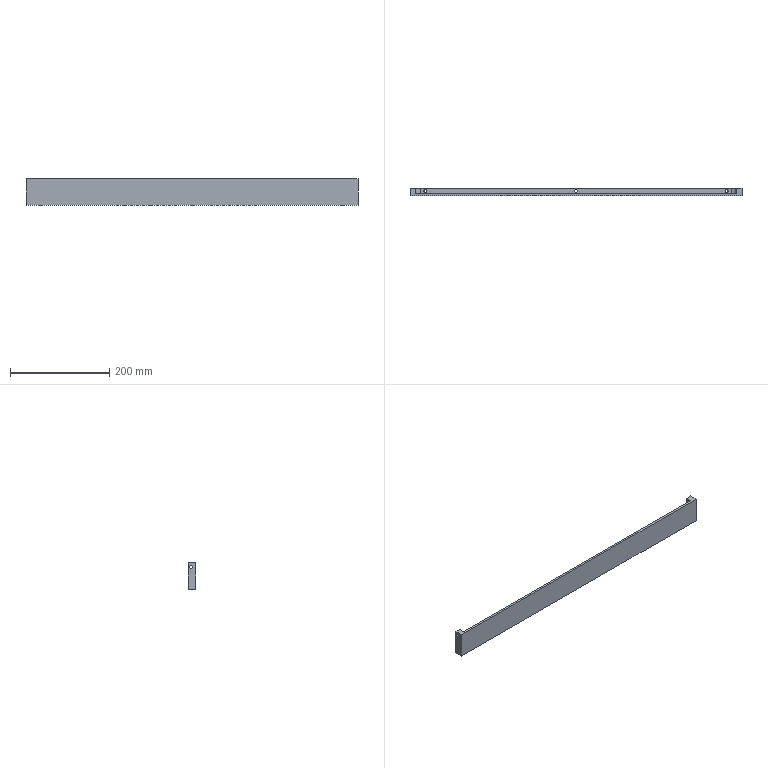Part | SolidWorks | features HoleWzd 2, MirrorPattern 2, Extrusion 1, Fillet 1, ICE 1 | 1 solid | 22 faces | box 670 x 16 x 52.685 mm | volume 357606 mm3 | cylinder 12 | plane 10 | commonest cylinder face diameters 6 x10 20 x2
STEP:
#1=CARTESIAN_POINT('',(-307.,10.,-26.343));
#2=VERTEX_POINT('',#1);
#3=CARTESIAN_POINT('',(-301.,10.,-26.343));
#4=VERTEX_POINT('',#3);
#5=CARTESIAN_POINT('',(-304.,10.,-26.343));
#6=DIRECTION('',(0.,0.,1.));
#7=DIRECTION('',(1.,0.,0.));
#8=AXIS2_PLACEMENT_3D('',#5,#6,#7);
#9=CIRCLE('',#8,3.);
#10=EDGE_CURVE('',#2,#4,#9,.T.);
#11=ORIENTED_EDGE('',*,*,#10,.F.);
#12=CARTESIAN_POINT('',(-307.,10.,0.));
#13=VERTEX_POINT('',#12);
#14=CARTESIAN_POINT('',(-307.,10.,0.));
#15=DIRECTION('',(0.,0.,1.));
#16=VECTOR('',#15,1000.);
#17=LINE('',#14,#16);
#18=EDGE_CURVE('',#2,#13,#17,.T.);
#19=ORIENTED_EDGE('',*,*,#18,.T.);
#20=CARTESIAN_POINT('',(-301.,10.,0.));
#21=VERTEX_POINT('',#20);
#22=CARTESIAN_POINT('',(-304.,10.,0.));
#23=DIRECTION('',(0.,0.,1.));
#24=DIRECTION('',(1.,0.,0.));
#25=AXIS2_PLACEMENT_3D('',#22,#23,#24);
#26=CIRCLE('',#25,3.);
#27=EDGE_CURVE('',#13,#21,#26,.T.);
#28=ORIENTED_EDGE('',*,*,#27,.T.);
#29=CARTESIAN_POINT('',(-301.,10.,0.));
#30=DIRECTION('',(0.,0.,1.));
#31=VECTOR('',#30,1000.);
#32=LINE('',#29,#31);
#33=EDGE_CURVE('',#4,#21,#32,.T.);
#34=ORIENTED_EDGE('',*,*,#33,.F.);
#35=EDGE_LOOP('',(#11,#19,#28,#34));
#36=FACE_OUTER_BOUND('',#35,.T.);
#37=CARTESIAN_POINT('',(-304.,10.,0.));
#38=DIRECTION('',(0.,0.,1.));
#39=DIRECTION('',(1.,0.,0.));
#40=AXIS2_PLACEMENT_3D('',#37,#38,#39);
#41=CYLINDRICAL_SURFACE('',#40,3.);
#42=ADVANCED_FACE('',(#36),#41,.F.);
#43=CARTESIAN_POINT('',(301.,10.,-26.343));
#44=VERTEX_POINT('',#43);
#45=CARTESIAN_POINT('',(307.,10.,-26.343));
#46=VERTEX_POINT('',#45);
#47=CARTESIAN_POINT('',(304.,10.,-26.343));
#48=DIRECTION('',(0.,0.,1.));
#49=DIRECTION('',(1.,0.,0.));
#50=AXIS2_PLACEMENT_3D('',#47,#48,#49);
#51=CIRCLE('',#50,3.);
#52=EDGE_CURVE('',#44,#46,#51,.T.);
#53=ORIENTED_EDGE('',*,*,#52,.F.);
#54=CARTESIAN_POINT('',(301.,10.,0.));
#55=VERTEX_POINT('',#54);
#56=CARTESIAN_POINT('',(301.,10.,0.));
#57=DIRECTION('',(0.,0.,1.));
#58=VECTOR('',#57,1000.);
#59=LINE('',#56,#58);
#60=EDGE_CURVE('',#44,#55,#59,.T.);
#61=ORIENTED_EDGE('',*,*,#60,.T.);
#62=CARTESIAN_POINT('',(307.,10.,0.));
#63=VERTEX_POINT('',#62);
#64=CARTESIAN_POINT('',(304.,10.,0.));
#65=DIRECTION('',(0.,0.,1.));
#66=DIRECTION('',(1.,0.,0.));
#67=AXIS2_PLACEMENT_3D('',#64,#65,#66);
#68=CIRCLE('',#67,3.);
#69=EDGE_CURVE('',#55,#63,#68,.T.);
#70=ORIENTED_EDGE('',*,*,#69,.T.);
#71=CARTESIAN_POINT('',(307.,10.,0.));
#72=DIRECTION('',(0.,0.,1.));
#73=VECTOR('',#72,1000.);
#74=LINE('',#71,#73);
#75=EDGE_CURVE('',#46,#63,#74,.T.);
#76=ORIENTED_EDGE('',*,*,#75,.F.);
#77=EDGE_LOOP('',(#53,#61,#70,#76));
#78=FACE_OUTER_BOUND('',#77,.T.);
#79=CARTESIAN_POINT('',(304.,10.,0.));
#80=DIRECTION('',(0.,0.,1.));
#81=DIRECTION('',(1.,0.,0.));
#82=AXIS2_PLACEMENT_3D('',#79,#80,#81);
#83=CYLINDRICAL_SURFACE('',#82,3.);
#84=ADVANCED_FACE('',(#78),#83,.F.);
#85=CARTESIAN_POINT('',(-3.,10.,-26.343));
#86=VERTEX_POINT('',#85);
#87=CARTESIAN_POINT('',(3.,10.,-26.343));
#88=VERTEX_POINT('',#87);
#89=CARTESIAN_POINT('',(0.,10.,-26.343));
#90=DIRECTION('',(0.,0.,1.));
#91=DIRECTION('',(1.,0.,0.));
#92=AXIS2_PLACEMENT_3D('',#89,#90,#91);
#93=CIRCLE('',#92,3.);
#94=EDGE_CURVE('',#86,#88,#93,.T.);
#95=ORIENTED_EDGE('',*,*,#94,.F.);
#96=CARTESIAN_POINT('',(-3.,10.,0.));
#97=VERTEX_POINT('',#96);
#98=CARTESIAN_POINT('',(-3.,10.,0.));
#99=DIRECTION('',(0.,0.,1.));
#100=VECTOR('',#99,1000.);
#101=LINE('',#98,#100);
#102=EDGE_CURVE('',#86,#97,#101,.T.);
#103=ORIENTED_EDGE('',*,*,#102,.T.);
#104=CARTESIAN_POINT('',(3.,10.,0.));
#105=VERTEX_POINT('',#104);
#106=CARTESIAN_POINT('',(0.,10.,0.));
#107=DIRECTION('',(0.,0.,1.));
#108=DIRECTION('',(1.,0.,0.));
#109=AXIS2_PLACEMENT_3D('',#106,#107,#108);
#110=CIRCLE('',#109,3.);
#111=EDGE_CURVE('',#97,#105,#110,.T.);
#112=ORIENTED_EDGE('',*,*,#111,.T.);
#113=CARTESIAN_POINT('',(3.,10.,0.));
#114=DIRECTION('',(0.,0.,1.));
#115=VECTOR('',#114,1000.);
#116=LINE('',#113,#115);
#117=EDGE_CURVE('',#88,#105,#116,.T.);
#118=ORIENTED_EDGE('',*,*,#117,.F.);
#119=EDGE_LOOP('',(#95,#103,#112,#118));
#120=FACE_OUTER_BOUND('',#119,.T.);
#121=CARTESIAN_POINT('',(0.,10.,0.));
#122=DIRECTION('',(0.,0.,1.));
#123=DIRECTION('',(1.,0.,0.));
#124=AXIS2_PLACEMENT_3D('',#121,#122,#123);
#125=CYLINDRICAL_SURFACE('',#124,3.);
#126=ADVANCED_FACE('',(#120),#125,.F.);
#127=CARTESIAN_POINT('',(-335.,10.,21.171));
#128=VERTEX_POINT('',#127);
#129=CARTESIAN_POINT('',(-335.,10.,15.171));
#130=VERTEX_POINT('',#129);
#131=CARTESIAN_POINT('',(-335.,10.,18.171));
#132=DIRECTION('',(1.,0.,0.));
#133=DIRECTION('',(0.,0.,-1.));
#134=AXIS2_PLACEMENT_3D('',#131,#132,#133);
#135=CIRCLE('',#134,3.);
#136=EDGE_CURVE('',#128,#130,#135,.T.);
#137=ORIENTED_EDGE('',*,*,#136,.F.);
#138=CARTESIAN_POINT('',(-324.,10.,21.171));
#139=VERTEX_POINT('',#138);
#140=CARTESIAN_POINT('',(-324.,10.,21.171));
#141=DIRECTION('',(1.,0.,0.));
#142=VECTOR('',#141,1000.);
#143=LINE('',#140,#142);
#144=EDGE_CURVE('',#128,#139,#143,.T.);
#145=ORIENTED_EDGE('',*,*,#144,.T.);
#146=CARTESIAN_POINT('',(-324.,10.,15.171));
#147=VERTEX_POINT('',#146);
#148=CARTESIAN_POINT('',(-324.,10.,18.171));
#149=DIRECTION('',(1.,0.,0.));
#150=DIRECTION('',(0.,0.,-1.));
#151=AXIS2_PLACEMENT_3D('',#148,#149,#150);
#152=CIRCLE('',#151,3.);
#153=EDGE_CURVE('',#139,#147,#152,.T.);
#154=ORIENTED_EDGE('',*,*,#153,.T.);
#155=CARTESIAN_POINT('',(-324.,10.,15.171));
#156=DIRECTION('',(1.,0.,0.));
#157=VECTOR('',#156,1000.);
#158=LINE('',#155,#157);
#159=EDGE_CURVE('',#130,#147,#158,.T.);
#160=ORIENTED_EDGE('',*,*,#159,.F.);
#161=EDGE_LOOP('',(#137,#145,#154,#160));
#162=FACE_OUTER_BOUND('',#161,.T.);
#163=CARTESIAN_POINT('',(-324.,10.,18.171));
#164=DIRECTION('',(1.,0.,0.));
#165=DIRECTION('',(0.,0.,-1.));
#166=AXIS2_PLACEMENT_3D('',#163,#164,#165);
#167=CYLINDRICAL_SURFACE('',#166,3.);
#168=ADVANCED_FACE('',(#162),#167,.F.);
#169=CARTESIAN_POINT('',(335.,10.,15.171));
#170=VERTEX_POINT('',#169);
#171=CARTESIAN_POINT('',(335.,10.,21.171));
#172=VERTEX_POINT('',#171);
#173=CARTESIAN_POINT('',(335.,10.,18.171));
#174=DIRECTION('',(-1.,0.,0.));
#175=DIRECTION('',(0.,0.,1.));
#176=AXIS2_PLACEMENT_3D('',#173,#174,#175);
#177=CIRCLE('',#176,3.);
#178=EDGE_CURVE('',#170,#172,#177,.T.);
#179=ORIENTED_EDGE('',*,*,#178,.F.);
#180=CARTESIAN_POINT('',(324.,10.,15.171));
#181=VERTEX_POINT('',#180);
#182=CARTESIAN_POINT('',(324.,10.,15.171));
#183=DIRECTION('',(-1.,0.,0.));
#184=VECTOR('',#183,1000.);
#185=LINE('',#182,#184);
#186=EDGE_CURVE('',#170,#181,#185,.T.);
#187=ORIENTED_EDGE('',*,*,#186,.T.);
#188=CARTESIAN_POINT('',(324.,10.,21.171));
#189=VERTEX_POINT('',#188);
#190=CARTESIAN_POINT('',(324.,10.,18.171));
#191=DIRECTION('',(-1.,0.,0.));
#192=DIRECTION('',(0.,0.,1.));
#193=AXIS2_PLACEMENT_3D('',#190,#191,#192);
#194=CIRCLE('',#193,3.);
#195=EDGE_CURVE('',#181,#189,#194,.T.);
#196=ORIENTED_EDGE('',*,*,#195,.T.);
#197=CARTESIAN_POINT('',(324.,10.,21.171));
#198=DIRECTION('',(-1.,0.,0.));
#199=VECTOR('',#198,1000.);
#200=LINE('',#197,#199);
#201=EDGE_CURVE('',#172,#189,#200,.T.);
#202=ORIENTED_EDGE('',*,*,#201,.F.);
#203=EDGE_LOOP('',(#179,#187,#196,#202));
#204=FACE_OUTER_BOUND('',#203,.T.);
#205=CARTESIAN_POINT('',(324.,10.,18.171));
#206=DIRECTION('',(-1.,0.,0.));
#207=DIRECTION('',(0.,0.,1.));
#208=AXIS2_PLACEMENT_3D('',#205,#206,#207);
#209=CYLINDRICAL_SURFACE('',#208,3.);
#210=ADVANCED_FACE('',(#204),#209,.F.);
#211=CARTESIAN_POINT('',(-335.,10.,18.171));
#212=DIRECTION('',(1.,0.,0.));
#213=DIRECTION('',(0.,0.,-1.));
#214=AXIS2_PLACEMENT_3D('',#211,#212,#213);
#215=CIRCLE('',#214,3.);
#216=EDGE_CURVE('',#130,#128,#215,.T.);
#217=ORIENTED_EDGE('',*,*,#216,.T.);
#218=ORIENTED_EDGE('',*,*,#136,.T.);
#219=EDGE_LOOP('',(#217,#218));
#220=FACE_BOUND('',#219,.T.);
#221=CARTESIAN_POINT('',(-335.,0.,-26.343));
#222=VERTEX_POINT('',#221);
#223=CARTESIAN_POINT('',(-335.,0.,26.343));
#224=VERTEX_POINT('',#223);
#225=CARTESIAN_POINT('',(-335.,0.,-26.343));
#226=DIRECTION('',(0.,0.,1.));
#227=VECTOR('',#226,1000.);
#228=LINE('',#225,#227);
#229=EDGE_CURVE('',#222,#224,#228,.T.);
#230=ORIENTED_EDGE('',*,*,#229,.T.);
#231=CARTESIAN_POINT('',(-335.,16.,26.343));
#232=VERTEX_POINT('',#231);
#233=CARTESIAN_POINT('',(-335.,16.,26.343));
#234=DIRECTION('',(0.,-1.,0.));
#235=VECTOR('',#234,1000.);
#236=LINE('',#233,#235);
#237=EDGE_CURVE('',#232,#224,#236,.T.);
#238=ORIENTED_EDGE('',*,*,#237,.F.);
#239=CARTESIAN_POINT('',(-335.,16.,-26.343));
#240=VERTEX_POINT('',#239);
#241=CARTESIAN_POINT('',(-335.,16.,-26.343));
#242=DIRECTION('',(0.,0.,1.));
#243=VECTOR('',#242,1000.);
#244=LINE('',#241,#243);
#245=EDGE_CURVE('',#240,#232,#244,.T.);
#246=ORIENTED_EDGE('',*,*,#245,.F.);
#247=CARTESIAN_POINT('',(-335.,16.,-26.343));
#248=DIRECTION('',(0.,-1.,0.));
#249=VECTOR('',#248,1000.);
#250=LINE('',#247,#249);
#251=EDGE_CURVE('',#240,#222,#250,.T.);
#252=ORIENTED_EDGE('',*,*,#251,.T.);
#253=EDGE_LOOP('',(#230,#238,#246,#252));
#254=FACE_OUTER_BOUND('',#253,.T.);
#255=CARTESIAN_POINT('',(-335.,16.,-26.343));
#256=DIRECTION('',(1.,0.,0.));
#257=DIRECTION('',(0.,0.,-1.));
#258=AXIS2_PLACEMENT_3D('',#255,#256,#257);
#259=PLANE('',#258);
#260=ADVANCED_FACE('',(#220,#254),#259,.F.);
#261=CARTESIAN_POINT('',(-324.,4.,26.343));
#262=VERTEX_POINT('',#261);
#263=CARTESIAN_POINT('',(324.,4.,26.343));
#264=VERTEX_POINT('',#263);
#265=CARTESIAN_POINT('',(335.,4.,26.343));
#266=DIRECTION('',(1.,0.,0.));
#267=VECTOR('',#266,1000.);
#268=LINE('',#265,#267);
#269=EDGE_CURVE('',#262,#264,#268,.T.);
#270=ORIENTED_EDGE('',*,*,#269,.F.);
#271=CARTESIAN_POINT('',(-324.,16.,26.343));
#272=VERTEX_POINT('',#271);
#273=CARTESIAN_POINT('',(-324.,16.,26.343));
#274=DIRECTION('',(0.,1.,0.));
#275=VECTOR('',#274,1000.);
#276=LINE('',#273,#275);
#277=EDGE_CURVE('',#262,#272,#276,.T.);
#278=ORIENTED_EDGE('',*,*,#277,.T.);
#279=CARTESIAN_POINT('',(335.,16.,26.343));
#280=DIRECTION('',(1.,0.,0.));
#281=VECTOR('',#280,1000.);
#282=LINE('',#279,#281);
#283=EDGE_CURVE('',#232,#272,#282,.T.);
#284=ORIENTED_EDGE('',*,*,#283,.F.);
#285=ORIENTED_EDGE('',*,*,#237,.T.);
#286=CARTESIAN_POINT('',(335.,0.,26.343));
#287=VERTEX_POINT('',#286);
#288=CARTESIAN_POINT('',(335.,0.,26.343));
#289=DIRECTION('',(1.,0.,0.));
#290=VECTOR('',#289,1000.);
#291=LINE('',#288,#290);
#292=EDGE_CURVE('',#224,#287,#291,.T.);
#293=ORIENTED_EDGE('',*,*,#292,.T.);
#294=CARTESIAN_POINT('',(335.,16.,26.343));
#295=VERTEX_POINT('',#294);
#296=CARTESIAN_POINT('',(335.,16.,26.343));
#297=DIRECTION('',(0.,-1.,0.));
#298=VECTOR('',#297,1000.);
#299=LINE('',#296,#298);
#300=EDGE_CURVE('',#295,#287,#299,.T.);
#301=ORIENTED_EDGE('',*,*,#300,.F.);
#302=CARTESIAN_POINT('',(324.,16.,26.343));
#303=VERTEX_POINT('',#302);
#304=CARTESIAN_POINT('',(335.,16.,26.343));
#305=DIRECTION('',(1.,0.,0.));
#306=VECTOR('',#305,1000.);
#307=LINE('',#304,#306);
#308=EDGE_CURVE('',#303,#295,#307,.T.);
#309=ORIENTED_EDGE('',*,*,#308,.F.);
#310=CARTESIAN_POINT('',(324.,16.,26.343));
#311=DIRECTION('',(0.,-1.,0.));
#312=VECTOR('',#311,1000.);
#313=LINE('',#310,#312);
#314=EDGE_CURVE('',#303,#264,#313,.T.);
#315=ORIENTED_EDGE('',*,*,#314,.T.);
#316=EDGE_LOOP('',(#270,#278,#284,#285,#293,#301,#309,#315));
#317=FACE_OUTER_BOUND('',#316,.T.);
#318=CARTESIAN_POINT('',(335.,16.,26.343));
#319=DIRECTION('',(0.,0.,-1.));
#320=DIRECTION('',(-1.,0.,0.));
#321=AXIS2_PLACEMENT_3D('',#318,#319,#320);
#322=PLANE('',#321);
#323=ADVANCED_FACE('',(#317),#322,.F.);
#324=CARTESIAN_POINT('',(335.,10.,18.171));
#325=DIRECTION('',(-1.,0.,0.));
#326=DIRECTION('',(0.,0.,1.));
#327=AXIS2_PLACEMENT_3D('',#324,#325,#326);
#328=CIRCLE('',#327,3.);
#329=EDGE_CURVE('',#172,#170,#328,.T.);
#330=ORIENTED_EDGE('',*,*,#329,.T.);
#331=ORIENTED_EDGE('',*,*,#178,.T.);
#332=EDGE_LOOP('',(#330,#331));
#333=FACE_BOUND('',#332,.T.);
#334=CARTESIAN_POINT('',(335.,0.,-26.343));
#335=VERTEX_POINT('',#334);
#336=CARTESIAN_POINT('',(335.,0.,-26.343));
#337=DIRECTION('',(0.,0.,-1.));
#338=VECTOR('',#337,1000.);
#339=LINE('',#336,#338);
#340=EDGE_CURVE('',#287,#335,#339,.T.);
#341=ORIENTED_EDGE('',*,*,#340,.T.);
#342=CARTESIAN_POINT('',(335.,16.,-26.343));
#343=VERTEX_POINT('',#342);
#344=CARTESIAN_POINT('',(335.,16.,-26.343));
#345=DIRECTION('',(0.,-1.,0.));
#346=VECTOR('',#345,1000.);
#347=LINE('',#344,#346);
#348=EDGE_CURVE('',#343,#335,#347,.T.);
#349=ORIENTED_EDGE('',*,*,#348,.F.);
#350=CARTESIAN_POINT('',(335.,16.,-26.343));
#351=DIRECTION('',(0.,0.,-1.));
#352=VECTOR('',#351,1000.);
#353=LINE('',#350,#352);
#354=EDGE_CURVE('',#295,#343,#353,.T.);
#355=ORIENTED_EDGE('',*,*,#354,.F.);
#356=ORIENTED_EDGE('',*,*,#300,.T.);
#357=EDGE_LOOP('',(#341,#349,#355,#356));
#358=FACE_OUTER_BOUND('',#357,.T.);
#359=CARTESIAN_POINT('',(335.,16.,-26.343));
#360=DIRECTION('',(-1.,0.,0.));
#361=DIRECTION('',(0.,0.,1.));
#362=AXIS2_PLACEMENT_3D('',#359,#360,#361);
#363=PLANE('',#362);
#364=ADVANCED_FACE('',(#333,#358),#363,.F.);
#365=CARTESIAN_POINT('',(-304.,10.,-26.343));
#366=DIRECTION('',(0.,0.,1.));
#367=DIRECTION('',(1.,0.,0.));
#368=AXIS2_PLACEMENT_3D('',#365,#366,#367);
#369=CIRCLE('',#368,3.);
#370=EDGE_CURVE('',#4,#2,#369,.T.);
#371=ORIENTED_EDGE('',*,*,#370,.T.);
#372=ORIENTED_EDGE('',*,*,#10,.T.);
#373=EDGE_LOOP('',(#371,#372));
#374=FACE_BOUND('',#373,.T.);
#375=CARTESIAN_POINT('',(304.,10.,-26.343));
#376=DIRECTION('',(0.,0.,1.));
#377=DIRECTION('',(1.,0.,0.));
#378=AXIS2_PLACEMENT_3D('',#375,#376,#377);
#379=CIRCLE('',#378,3.);
#380=EDGE_CURVE('',#46,#44,#379,.T.);
#381=ORIENTED_EDGE('',*,*,#380,.T.);
#382=ORIENTED_EDGE('',*,*,#52,.T.);
#383=EDGE_LOOP('',(#381,#382));
#384=FACE_BOUND('',#383,.T.);
#385=CARTESIAN_POINT('',(0.,10.,-26.343));
#386=DIRECTION('',(0.,0.,1.));
#387=DIRECTION('',(1.,0.,0.));
#388=AXIS2_PLACEMENT_3D('',#385,#386,#387);
#389=CIRCLE('',#388,3.);
#390=EDGE_CURVE('',#88,#86,#389,.T.);
#391=ORIENTED_EDGE('',*,*,#390,.T.);
#392=ORIENTED_EDGE('',*,*,#94,.T.);
#393=EDGE_LOOP('',(#391,#392));
#394=FACE_BOUND('',#393,.T.);
#395=CARTESIAN_POINT('',(335.,0.,-26.343));
#396=DIRECTION('',(-1.,0.,0.));
#397=VECTOR('',#396,1000.);
#398=LINE('',#395,#397);
#399=EDGE_CURVE('',#335,#222,#398,.T.);
#400=ORIENTED_EDGE('',*,*,#399,.T.);
#401=ORIENTED_EDGE('',*,*,#251,.F.);
#402=CARTESIAN_POINT('',(335.,16.,-26.343));
#403=DIRECTION('',(-1.,0.,0.));
#404=VECTOR('',#403,1000.);
#405=LINE('',#402,#404);
#406=EDGE_CURVE('',#343,#240,#405,.T.);
#407=ORIENTED_EDGE('',*,*,#406,.F.);
#408=ORIENTED_EDGE('',*,*,#348,.T.);
#409=EDGE_LOOP('',(#400,#401,#407,#408));
#410=FACE_OUTER_BOUND('',#409,.T.);
#411=CARTESIAN_POINT('',(335.,16.,-26.343));
#412=DIRECTION('',(0.,0.,1.));
#413=DIRECTION('',(1.,0.,0.));
#414=AXIS2_PLACEMENT_3D('',#411,#412,#413);
#415=PLANE('',#414);
#416=ADVANCED_FACE('',(#374,#384,#394,#410),#415,.F.);
#417=ORIENTED_EDGE('',*,*,#283,.T.);
#418=CARTESIAN_POINT('',(-324.,16.,10.));
#419=VERTEX_POINT('',#418);
#420=CARTESIAN_POINT('',(-324.,16.,0.));
#421=DIRECTION('',(0.,0.,1.));
#422=VECTOR('',#421,1000.);
#423=LINE('',#420,#422);
#424=EDGE_CURVE('',#419,#272,#423,.T.);
#425=ORIENTED_EDGE('',*,*,#424,.F.);
#426=CARTESIAN_POINT('',(-314.,16.,0.));
#427=VERTEX_POINT('',#426);
#428=CARTESIAN_POINT('',(-314.,16.,10.));
#429=DIRECTION('',(0.,-1.,0.));
#430=DIRECTION('',(0.,0.,-1.));
#431=AXIS2_PLACEMENT_3D('',#428,#429,#430);
#432=CIRCLE('',#431,10.);
#433=EDGE_CURVE('',#419,#427,#432,.T.);
#434=ORIENTED_EDGE('',*,*,#433,.T.);
#435=CARTESIAN_POINT('',(314.,16.,0.));
#436=VERTEX_POINT('',#435);
#437=CARTESIAN_POINT('',(-324.,16.,0.));
#438=DIRECTION('',(-1.,0.,0.));
#439=VECTOR('',#438,1000.);
#440=LINE('',#437,#439);
#441=EDGE_CURVE('',#436,#427,#440,.T.);
#442=ORIENTED_EDGE('',*,*,#441,.F.);
#443=CARTESIAN_POINT('',(324.,16.,10.));
#444=VERTEX_POINT('',#443);
#445=CARTESIAN_POINT('',(314.,16.,10.));
#446=DIRECTION('',(0.,-1.,0.));
#447=DIRECTION('',(0.,0.,-1.));
#448=AXIS2_PLACEMENT_3D('',#445,#446,#447);
#449=CIRCLE('',#448,10.);
#450=EDGE_CURVE('',#436,#444,#449,.T.);
#451=ORIENTED_EDGE('',*,*,#450,.T.);
#452=CARTESIAN_POINT('',(324.,16.,0.));
#453=DIRECTION('',(0.,0.,1.));
#454=VECTOR('',#453,1000.);
#455=LINE('',#452,#454);
#456=EDGE_CURVE('',#444,#303,#455,.T.);
#457=ORIENTED_EDGE('',*,*,#456,.T.);
#458=ORIENTED_EDGE('',*,*,#308,.T.);
#459=ORIENTED_EDGE('',*,*,#354,.T.);
#460=ORIENTED_EDGE('',*,*,#406,.T.);
#461=ORIENTED_EDGE('',*,*,#245,.T.);
#462=EDGE_LOOP('',(#417,#425,#434,#442,#451,#457,#458,#459,#460,#461));
#463=FACE_OUTER_BOUND('',#462,.T.);
#464=CARTESIAN_POINT('',(0.,16.,0.));
#465=DIRECTION('',(0.,-1.,0.));
#466=DIRECTION('',(0.,0.,-1.));
#467=AXIS2_PLACEMENT_3D('',#464,#465,#466);
#468=PLANE('',#467);
#469=ADVANCED_FACE('',(#463),#468,.F.);
#470=ORIENTED_EDGE('',*,*,#229,.F.);
#471=ORIENTED_EDGE('',*,*,#399,.F.);
#472=ORIENTED_EDGE('',*,*,#340,.F.);
#473=ORIENTED_EDGE('',*,*,#292,.F.);
#474=EDGE_LOOP('',(#470,#471,#472,#473));
#475=FACE_OUTER_BOUND('',#474,.T.);
#476=CARTESIAN_POINT('',(0.,0.,0.));
#477=DIRECTION('',(0.,-1.,0.));
#478=DIRECTION('',(0.,0.,-1.));
#479=AXIS2_PLACEMENT_3D('',#476,#477,#478);
#480=PLANE('',#479);
#481=ADVANCED_FACE('',(#475),#480,.T.);
#482=CARTESIAN_POINT('',(324.,4.,10.));
#483=VERTEX_POINT('',#482);
#484=CARTESIAN_POINT('',(324.,4.,0.));
#485=DIRECTION('',(0.,0.,-1.));
#486=VECTOR('',#485,1000.);
#487=LINE('',#484,#486);
#488=EDGE_CURVE('',#264,#483,#487,.T.);
#489=ORIENTED_EDGE('',*,*,#488,.T.);
#490=CARTESIAN_POINT('',(314.,4.,0.));
#491=VERTEX_POINT('',#490);
#492=CARTESIAN_POINT('',(314.,4.,10.));
#493=DIRECTION('',(0.,1.,0.));
#494=DIRECTION('',(0.,0.,1.));
#495=AXIS2_PLACEMENT_3D('',#492,#493,#494);
#496=CIRCLE('',#495,10.);
#497=EDGE_CURVE('',#483,#491,#496,.T.);
#498=ORIENTED_EDGE('',*,*,#497,.T.);
#499=CARTESIAN_POINT('',(-314.,4.,0.));
#500=VERTEX_POINT('',#499);
#501=CARTESIAN_POINT('',(-324.,4.,0.));
#502=DIRECTION('',(-1.,0.,0.));
#503=VECTOR('',#502,1000.);
#504=LINE('',#501,#503);
#505=EDGE_CURVE('',#491,#500,#504,.T.);
#506=ORIENTED_EDGE('',*,*,#505,.T.);
#507=CARTESIAN_POINT('',(-324.,4.,10.));
#508=VERTEX_POINT('',#507);
#509=CARTESIAN_POINT('',(-314.,4.,10.));
#510=DIRECTION('',(0.,1.,0.));
#511=DIRECTION('',(0.,0.,1.));
#512=AXIS2_PLACEMENT_3D('',#509,#510,#511);
#513=CIRCLE('',#512,10.);
#514=EDGE_CURVE('',#500,#508,#513,.T.);
#515=ORIENTED_EDGE('',*,*,#514,.T.);
#516=CARTESIAN_POINT('',(-324.,4.,0.));
#517=DIRECTION('',(0.,0.,1.));
#518=VECTOR('',#517,1000.);
#519=LINE('',#516,#518);
#520=EDGE_CURVE('',#508,#262,#519,.T.);
#521=ORIENTED_EDGE('',*,*,#520,.T.);
#522=ORIENTED_EDGE('',*,*,#269,.T.);
#523=EDGE_LOOP('',(#489,#498,#506,#515,#521,#522));
#524=FACE_OUTER_BOUND('',#523,.T.);
#525=CARTESIAN_POINT('',(0.,4.,0.));
#526=DIRECTION('',(0.,1.,0.));
#527=DIRECTION('',(0.,0.,1.));
#528=AXIS2_PLACEMENT_3D('',#525,#526,#527);
#529=PLANE('',#528);
#530=ADVANCED_FACE('',(#524),#529,.T.);
#531=CARTESIAN_POINT('',(-324.,10.,18.171));
#532=DIRECTION('',(1.,0.,0.));
#533=DIRECTION('',(0.,0.,-1.));
#534=AXIS2_PLACEMENT_3D('',#531,#532,#533);
#535=CIRCLE('',#534,3.);
#536=EDGE_CURVE('',#147,#139,#535,.T.);
#537=ORIENTED_EDGE('',*,*,#536,.F.);
#538=ORIENTED_EDGE('',*,*,#153,.F.);
#539=EDGE_LOOP('',(#537,#538));
#540=FACE_BOUND('',#539,.T.);
#541=ORIENTED_EDGE('',*,*,#520,.F.);
#542=CARTESIAN_POINT('',(-324.,16.,10.));
#543=DIRECTION('',(0.,1.,0.));
#544=VECTOR('',#543,1000.);
#545=LINE('',#542,#544);
#546=EDGE_CURVE('',#508,#419,#545,.T.);
#547=ORIENTED_EDGE('',*,*,#546,.T.);
#548=ORIENTED_EDGE('',*,*,#424,.T.);
#549=ORIENTED_EDGE('',*,*,#277,.F.);
#550=EDGE_LOOP('',(#541,#547,#548,#549));
#551=FACE_OUTER_BOUND('',#550,.T.);
#552=CARTESIAN_POINT('',(-324.,4.,0.));
#553=DIRECTION('',(-1.,0.,0.));
#554=DIRECTION('',(0.,0.,1.));
#555=AXIS2_PLACEMENT_3D('',#552,#553,#554);
#556=PLANE('',#555);
#557=ADVANCED_FACE('',(#540,#551),#556,.F.);
#558=CARTESIAN_POINT('',(324.,10.,18.171));
#559=DIRECTION('',(-1.,0.,0.));
#560=DIRECTION('',(0.,0.,1.));
#561=AXIS2_PLACEMENT_3D('',#558,#559,#560);
#562=CIRCLE('',#561,3.);
#563=EDGE_CURVE('',#189,#181,#562,.T.);
#564=ORIENTED_EDGE('',*,*,#563,.F.);
#565=ORIENTED_EDGE('',*,*,#195,.F.);
#566=EDGE_LOOP('',(#564,#565));
#567=FACE_BOUND('',#566,.T.);
#568=ORIENTED_EDGE('',*,*,#456,.F.);
#569=CARTESIAN_POINT('',(324.,4.,10.));
#570=DIRECTION('',(0.,-1.,0.));
#571=VECTOR('',#570,1000.);
#572=LINE('',#569,#571);
#573=EDGE_CURVE('',#444,#483,#572,.T.);
#574=ORIENTED_EDGE('',*,*,#573,.T.);
#575=ORIENTED_EDGE('',*,*,#488,.F.);
#576=ORIENTED_EDGE('',*,*,#314,.F.);
#577=EDGE_LOOP('',(#568,#574,#575,#576));
#578=FACE_OUTER_BOUND('',#577,.T.);
#579=CARTESIAN_POINT('',(324.,4.,0.));
#580=DIRECTION('',(1.,0.,0.));
#581=DIRECTION('',(0.,0.,-1.));
#582=AXIS2_PLACEMENT_3D('',#579,#580,#581);
#583=PLANE('',#582);
#584=ADVANCED_FACE('',(#567,#578),#583,.F.);
#585=CARTESIAN_POINT('',(-304.,10.,0.));
#586=DIRECTION('',(0.,0.,1.));
#587=DIRECTION('',(1.,0.,0.));
#588=AXIS2_PLACEMENT_3D('',#585,#586,#587);
#589=CIRCLE('',#588,3.);
#590=EDGE_CURVE('',#21,#13,#589,.T.);
#591=ORIENTED_EDGE('',*,*,#590,.F.);
#592=ORIENTED_EDGE('',*,*,#27,.F.);
#593=EDGE_LOOP('',(#591,#592));
#594=FACE_BOUND('',#593,.T.);
#595=CARTESIAN_POINT('',(304.,10.,0.));
#596=DIRECTION('',(0.,0.,1.));
#597=DIRECTION('',(1.,0.,0.));
#598=AXIS2_PLACEMENT_3D('',#595,#596,#597);
#599=CIRCLE('',#598,3.);
#600=EDGE_CURVE('',#63,#55,#599,.T.);
#601=ORIENTED_EDGE('',*,*,#600,.F.);
#602=ORIENTED_EDGE('',*,*,#69,.F.);
#603=EDGE_LOOP('',(#601,#602));
#604=FACE_BOUND('',#603,.T.);
#605=CARTESIAN_POINT('',(0.,10.,0.));
#606=DIRECTION('',(0.,0.,1.));
#607=DIRECTION('',(1.,0.,0.));
#608=AXIS2_PLACEMENT_3D('',#605,#606,#607);
#609=CIRCLE('',#608,3.);
#610=EDGE_CURVE('',#105,#97,#609,.T.);
#611=ORIENTED_EDGE('',*,*,#610,.F.);
#612=ORIENTED_EDGE('',*,*,#111,.F.);
#613=EDGE_LOOP('',(#611,#612));
#614=FACE_BOUND('',#613,.T.);
#615=ORIENTED_EDGE('',*,*,#505,.F.);
#616=CARTESIAN_POINT('',(314.,16.,0.));
#617=DIRECTION('',(0.,1.,0.));
#618=VECTOR('',#617,1000.);
#619=LINE('',#616,#618);
#620=EDGE_CURVE('',#491,#436,#619,.T.);
#621=ORIENTED_EDGE('',*,*,#620,.T.);
#622=ORIENTED_EDGE('',*,*,#441,.T.);
#623=CARTESIAN_POINT('',(-314.,4.,0.));
#624=DIRECTION('',(0.,-1.,0.));
#625=VECTOR('',#624,1000.);
#626=LINE('',#623,#625);
#627=EDGE_CURVE('',#427,#500,#626,.T.);
#628=ORIENTED_EDGE('',*,*,#627,.T.);
#629=EDGE_LOOP('',(#615,#621,#622,#628));
#630=FACE_OUTER_BOUND('',#629,.T.);
#631=CARTESIAN_POINT('',(-324.,4.,0.));
#632=DIRECTION('',(0.,0.,-1.));
#633=DIRECTION('',(-1.,0.,0.));
#634=AXIS2_PLACEMENT_3D('',#631,#632,#633);
#635=PLANE('',#634);
#636=ADVANCED_FACE('',(#594,#604,#614,#630),#635,.F.);
#637=ORIENTED_EDGE('',*,*,#497,.F.);
#638=ORIENTED_EDGE('',*,*,#573,.F.);
#639=ORIENTED_EDGE('',*,*,#450,.F.);
#640=ORIENTED_EDGE('',*,*,#620,.F.);
#641=EDGE_LOOP('',(#637,#638,#639,#640));
#642=FACE_OUTER_BOUND('',#641,.T.);
#643=CARTESIAN_POINT('',(314.,4.,10.));
#644=DIRECTION('',(0.,-1.,0.));
#645=DIRECTION('',(0.,0.,-1.));
#646=AXIS2_PLACEMENT_3D('',#643,#644,#645);
#647=CYLINDRICAL_SURFACE('',#646,10.);
#648=ADVANCED_FACE('',(#642),#647,.F.);
#649=ORIENTED_EDGE('',*,*,#514,.F.);
#650=ORIENTED_EDGE('',*,*,#627,.F.);
#651=ORIENTED_EDGE('',*,*,#433,.F.);
#652=ORIENTED_EDGE('',*,*,#546,.F.);
#653=EDGE_LOOP('',(#649,#650,#651,#652));
#654=FACE_OUTER_BOUND('',#653,.T.);
#655=CARTESIAN_POINT('',(-314.,4.,10.));
#656=DIRECTION('',(0.,-1.,0.));
#657=DIRECTION('',(0.,0.,-1.));
#658=AXIS2_PLACEMENT_3D('',#655,#656,#657);
#659=CYLINDRICAL_SURFACE('',#658,10.);
#660=ADVANCED_FACE('',(#654),#659,.F.);
#661=ORIENTED_EDGE('',*,*,#186,.F.);
#662=ORIENTED_EDGE('',*,*,#329,.F.);
#663=ORIENTED_EDGE('',*,*,#201,.T.);
#664=ORIENTED_EDGE('',*,*,#563,.T.);
#665=EDGE_LOOP('',(#661,#662,#663,#664));
#666=FACE_OUTER_BOUND('',#665,.T.);
#667=CARTESIAN_POINT('',(324.,10.,18.171));
#668=DIRECTION('',(-1.,0.,0.));
#669=DIRECTION('',(0.,0.,1.));
#670=AXIS2_PLACEMENT_3D('',#667,#668,#669);
#671=CYLINDRICAL_SURFACE('',#670,3.);
#672=ADVANCED_FACE('',(#666),#671,.F.);
#673=ORIENTED_EDGE('',*,*,#144,.F.);
#674=ORIENTED_EDGE('',*,*,#216,.F.);
#675=ORIENTED_EDGE('',*,*,#159,.T.);
#676=ORIENTED_EDGE('',*,*,#536,.T.);
#677=EDGE_LOOP('',(#673,#674,#675,#676));
#678=FACE_OUTER_BOUND('',#677,.T.);
#679=CARTESIAN_POINT('',(-324.,10.,18.171));
#680=DIRECTION('',(1.,0.,0.));
#681=DIRECTION('',(0.,0.,-1.));
#682=AXIS2_PLACEMENT_3D('',#679,#680,#681);
#683=CYLINDRICAL_SURFACE('',#682,3.);
#684=ADVANCED_FACE('',(#678),#683,.F.);
#685=ORIENTED_EDGE('',*,*,#102,.F.);
#686=ORIENTED_EDGE('',*,*,#390,.F.);
#687=ORIENTED_EDGE('',*,*,#117,.T.);
#688=ORIENTED_EDGE('',*,*,#610,.T.);
#689=EDGE_LOOP('',(#685,#686,#687,#688));
#690=FACE_OUTER_BOUND('',#689,.T.);
#691=CARTESIAN_POINT('',(0.,10.,0.));
#692=DIRECTION('',(0.,0.,1.));
#693=DIRECTION('',(1.,0.,0.));
#694=AXIS2_PLACEMENT_3D('',#691,#692,#693);
#695=CYLINDRICAL_SURFACE('',#694,3.);
#696=ADVANCED_FACE('',(#690),#695,.F.);
#697=ORIENTED_EDGE('',*,*,#60,.F.);
#698=ORIENTED_EDGE('',*,*,#380,.F.);
#699=ORIENTED_EDGE('',*,*,#75,.T.);
#700=ORIENTED_EDGE('',*,*,#600,.T.);
#701=EDGE_LOOP('',(#697,#698,#699,#700));
#702=FACE_OUTER_BOUND('',#701,.T.);
#703=CARTESIAN_POINT('',(304.,10.,0.));
#704=DIRECTION('',(0.,0.,1.));
#705=DIRECTION('',(1.,0.,0.));
#706=AXIS2_PLACEMENT_3D('',#703,#704,#705);
#707=CYLINDRICAL_SURFACE('',#706,3.);
#708=ADVANCED_FACE('',(#702),#707,.F.);
#709=ORIENTED_EDGE('',*,*,#18,.F.);
#710=ORIENTED_EDGE('',*,*,#370,.F.);
#711=ORIENTED_EDGE('',*,*,#33,.T.);
#712=ORIENTED_EDGE('',*,*,#590,.T.);
#713=EDGE_LOOP('',(#709,#710,#711,#712));
#714=FACE_OUTER_BOUND('',#713,.T.);
#715=CARTESIAN_POINT('',(-304.,10.,0.));
#716=DIRECTION('',(0.,0.,1.));
#717=DIRECTION('',(1.,0.,0.));
#718=AXIS2_PLACEMENT_3D('',#715,#716,#717);
#719=CYLINDRICAL_SURFACE('',#718,3.);
#720=ADVANCED_FACE('',(#714),#719,.F.);
#721=CLOSED_SHELL('',(#42,#84,#126,#168,#210,#260,#323,#364,#416,#469,#481,#530,#557,#584,#636,#648,#660,#672,#684,#696,#708,#720));
#722=MANIFOLD_SOLID_BREP('',#721);
#723=CARTESIAN_POINT('',(0.,0.,0.));
#724=DIRECTION('',(0.,0.,1.));
#725=DIRECTION('',(1.,0.,0.));
#726=AXIS2_PLACEMENT_3D('',#723,#724,#725);
#727=(LENGTH_UNIT()NAMED_UNIT(*)SI_UNIT(.MILLI.,.METRE.));
#728=UNCERTAINTY_MEASURE_WITH_UNIT(LENGTH_MEASURE(0.00001),#727,'','');
#729=(NAMED_UNIT(*)PLANE_ANGLE_UNIT()SI_UNIT($,.RADIAN.));
#730=(NAMED_UNIT(*)SI_UNIT($,.STERADIAN.)SOLID_ANGLE_UNIT());
#731=(GEOMETRIC_REPRESENTATION_CONTEXT(3)GLOBAL_UNCERTAINTY_ASSIGNED_CONTEXT((#728))GLOBAL_UNIT_ASSIGNED_CONTEXT((#727,#729,#730))REPRESENTATION_CONTEXT('',''));
#732=ADVANCED_BREP_SHAPE_REPRESENTATION('',(#722,#726),#731);